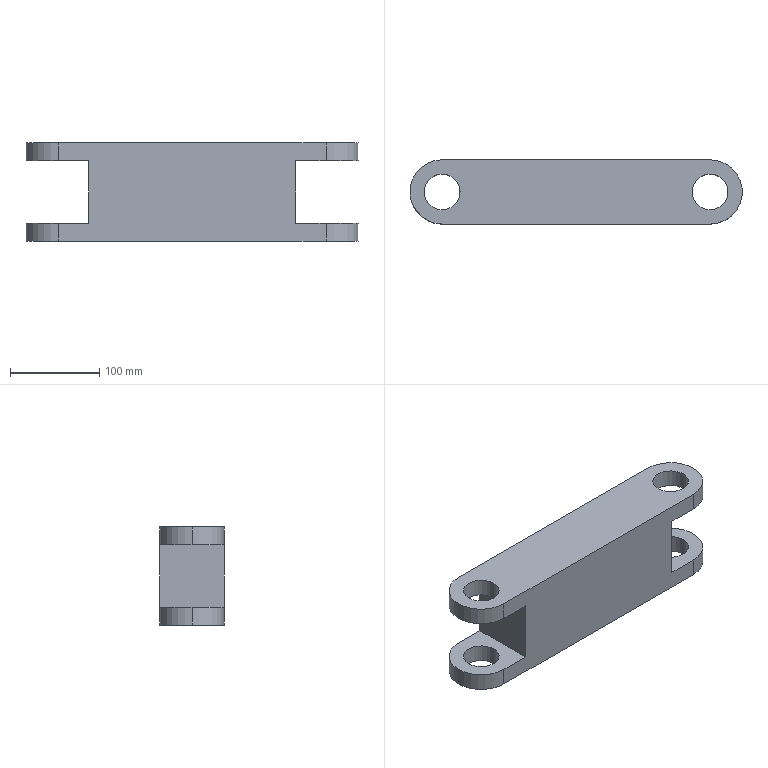Part | SolidWorks | 1 solid | 24 faces | box 372 x 72 x 110 mm | volume 2095609 mm3 | cylinder 14 | plane 10 | commonest cylinder face diameters 40 x8 72 x6
STEP:
#1=CARTESIAN_POINT('',(320.,0.,-35.));
#2=VERTEX_POINT('',#1);
#3=CARTESIAN_POINT('',(280.,0.,-35.));
#4=VERTEX_POINT('',#3);
#5=CARTESIAN_POINT('',(300.,0.,-35.));
#6=DIRECTION('',(0.,0.,-1.));
#7=DIRECTION('',(-1.,0.,0.));
#8=AXIS2_PLACEMENT_3D('',#5,#6,#7);
#9=CIRCLE('',#8,20.);
#10=EDGE_CURVE('',#2,#4,#9,.T.);
#11=ORIENTED_EDGE('',*,*,#10,.F.);
#12=CARTESIAN_POINT('',(320.,0.,-55.));
#13=VERTEX_POINT('',#12);
#14=CARTESIAN_POINT('',(320.,0.,55.));
#15=DIRECTION('',(0.,0.,-1.));
#16=VECTOR('',#15,1000.);
#17=LINE('',#14,#16);
#18=EDGE_CURVE('',#2,#13,#17,.T.);
#19=ORIENTED_EDGE('',*,*,#18,.T.);
#20=CARTESIAN_POINT('',(280.,0.,-55.));
#21=VERTEX_POINT('',#20);
#22=CARTESIAN_POINT('',(300.,0.,-55.));
#23=DIRECTION('',(0.,0.,1.));
#24=DIRECTION('',(1.,0.,0.));
#25=AXIS2_PLACEMENT_3D('',#22,#23,#24);
#26=CIRCLE('',#25,20.);
#27=EDGE_CURVE('',#21,#13,#26,.T.);
#28=ORIENTED_EDGE('',*,*,#27,.F.);
#29=CARTESIAN_POINT('',(280.,0.,55.));
#30=DIRECTION('',(0.,0.,-1.));
#31=VECTOR('',#30,1000.);
#32=LINE('',#29,#31);
#33=EDGE_CURVE('',#4,#21,#32,.T.);
#34=ORIENTED_EDGE('',*,*,#33,.F.);
#35=EDGE_LOOP('',(#11,#19,#28,#34));
#36=FACE_OUTER_BOUND('',#35,.T.);
#37=CARTESIAN_POINT('',(300.,0.,55.));
#38=DIRECTION('',(0.,0.,-1.));
#39=DIRECTION('',(-1.,0.,0.));
#40=AXIS2_PLACEMENT_3D('',#37,#38,#39);
#41=CYLINDRICAL_SURFACE('',#40,20.);
#42=ADVANCED_FACE('',(#36),#41,.F.);
#43=CARTESIAN_POINT('',(20.,0.,-35.));
#44=VERTEX_POINT('',#43);
#45=CARTESIAN_POINT('',(-20.,0.,-35.));
#46=VERTEX_POINT('',#45);
#47=CARTESIAN_POINT('',(0.,0.,-35.));
#48=DIRECTION('',(0.,0.,-1.));
#49=DIRECTION('',(-1.,0.,0.));
#50=AXIS2_PLACEMENT_3D('',#47,#48,#49);
#51=CIRCLE('',#50,20.);
#52=EDGE_CURVE('',#44,#46,#51,.T.);
#53=ORIENTED_EDGE('',*,*,#52,.F.);
#54=CARTESIAN_POINT('',(20.,0.,-55.));
#55=VERTEX_POINT('',#54);
#56=CARTESIAN_POINT('',(20.,0.,55.));
#57=DIRECTION('',(0.,0.,-1.));
#58=VECTOR('',#57,1000.);
#59=LINE('',#56,#58);
#60=EDGE_CURVE('',#44,#55,#59,.T.);
#61=ORIENTED_EDGE('',*,*,#60,.T.);
#62=CARTESIAN_POINT('',(-20.,0.,-55.));
#63=VERTEX_POINT('',#62);
#64=CARTESIAN_POINT('',(0.,0.,-55.));
#65=DIRECTION('',(0.,0.,1.));
#66=DIRECTION('',(1.,0.,0.));
#67=AXIS2_PLACEMENT_3D('',#64,#65,#66);
#68=CIRCLE('',#67,20.);
#69=EDGE_CURVE('',#63,#55,#68,.T.);
#70=ORIENTED_EDGE('',*,*,#69,.F.);
#71=CARTESIAN_POINT('',(-20.,0.,55.));
#72=DIRECTION('',(0.,0.,-1.));
#73=VECTOR('',#72,1000.);
#74=LINE('',#71,#73);
#75=EDGE_CURVE('',#46,#63,#74,.T.);
#76=ORIENTED_EDGE('',*,*,#75,.F.);
#77=EDGE_LOOP('',(#53,#61,#70,#76));
#78=FACE_OUTER_BOUND('',#77,.T.);
#79=CARTESIAN_POINT('',(0.,0.,55.));
#80=DIRECTION('',(0.,0.,-1.));
#81=DIRECTION('',(-1.,0.,0.));
#82=AXIS2_PLACEMENT_3D('',#79,#80,#81);
#83=CYLINDRICAL_SURFACE('',#82,20.);
#84=ADVANCED_FACE('',(#78),#83,.F.);
#85=CARTESIAN_POINT('',(0.,-36.,-35.));
#86=VERTEX_POINT('',#85);
#87=CARTESIAN_POINT('',(-36.,0.,-35.));
#88=VERTEX_POINT('',#87);
#89=CARTESIAN_POINT('',(0.,0.,-35.));
#90=DIRECTION('',(0.,0.,-1.));
#91=DIRECTION('',(-1.,0.,0.));
#92=AXIS2_PLACEMENT_3D('',#89,#90,#91);
#93=CIRCLE('',#92,36.);
#94=EDGE_CURVE('',#86,#88,#93,.T.);
#95=ORIENTED_EDGE('',*,*,#94,.T.);
#96=CARTESIAN_POINT('',(-36.,0.,-55.));
#97=VERTEX_POINT('',#96);
#98=CARTESIAN_POINT('',(-36.,0.,55.));
#99=DIRECTION('',(0.,0.,-1.));
#100=VECTOR('',#99,1000.);
#101=LINE('',#98,#100);
#102=EDGE_CURVE('',#88,#97,#101,.T.);
#103=ORIENTED_EDGE('',*,*,#102,.T.);
#104=CARTESIAN_POINT('',(0.,-36.,-55.));
#105=VERTEX_POINT('',#104);
#106=CARTESIAN_POINT('',(0.,0.,-55.));
#107=DIRECTION('',(0.,0.,1.));
#108=DIRECTION('',(1.,0.,0.));
#109=AXIS2_PLACEMENT_3D('',#106,#107,#108);
#110=CIRCLE('',#109,36.);
#111=EDGE_CURVE('',#97,#105,#110,.T.);
#112=ORIENTED_EDGE('',*,*,#111,.T.);
#113=CARTESIAN_POINT('',(0.,-36.,55.));
#114=DIRECTION('',(0.,0.,-1.));
#115=VECTOR('',#114,1000.);
#116=LINE('',#113,#115);
#117=EDGE_CURVE('',#86,#105,#116,.T.);
#118=ORIENTED_EDGE('',*,*,#117,.F.);
#119=EDGE_LOOP('',(#95,#103,#112,#118));
#120=FACE_OUTER_BOUND('',#119,.T.);
#121=CARTESIAN_POINT('',(0.,0.,55.));
#122=DIRECTION('',(0.,0.,-1.));
#123=DIRECTION('',(-1.,0.,0.));
#124=AXIS2_PLACEMENT_3D('',#121,#122,#123);
#125=CYLINDRICAL_SURFACE('',#124,36.);
#126=ADVANCED_FACE('',(#120),#125,.T.);
#127=CARTESIAN_POINT('',(280.,0.,55.));
#128=VERTEX_POINT('',#127);
#129=CARTESIAN_POINT('',(320.,0.,55.));
#130=VERTEX_POINT('',#129);
#131=CARTESIAN_POINT('',(300.,0.,55.));
#132=DIRECTION('',(0.,0.,1.));
#133=DIRECTION('',(1.,0.,0.));
#134=AXIS2_PLACEMENT_3D('',#131,#132,#133);
#135=CIRCLE('',#134,20.);
#136=EDGE_CURVE('',#128,#130,#135,.T.);
#137=ORIENTED_EDGE('',*,*,#136,.T.);
#138=CARTESIAN_POINT('',(320.,0.,35.));
#139=VERTEX_POINT('',#138);
#140=CARTESIAN_POINT('',(320.,0.,55.));
#141=DIRECTION('',(0.,0.,-1.));
#142=VECTOR('',#141,1000.);
#143=LINE('',#140,#142);
#144=EDGE_CURVE('',#130,#139,#143,.T.);
#145=ORIENTED_EDGE('',*,*,#144,.T.);
#146=CARTESIAN_POINT('',(280.,0.,35.));
#147=VERTEX_POINT('',#146);
#148=CARTESIAN_POINT('',(300.,0.,35.));
#149=DIRECTION('',(0.,0.,1.));
#150=DIRECTION('',(1.,0.,0.));
#151=AXIS2_PLACEMENT_3D('',#148,#149,#150);
#152=CIRCLE('',#151,20.);
#153=EDGE_CURVE('',#147,#139,#152,.T.);
#154=ORIENTED_EDGE('',*,*,#153,.F.);
#155=CARTESIAN_POINT('',(280.,0.,55.));
#156=DIRECTION('',(0.,0.,-1.));
#157=VECTOR('',#156,1000.);
#158=LINE('',#155,#157);
#159=EDGE_CURVE('',#128,#147,#158,.T.);
#160=ORIENTED_EDGE('',*,*,#159,.F.);
#161=EDGE_LOOP('',(#137,#145,#154,#160));
#162=FACE_OUTER_BOUND('',#161,.T.);
#163=CARTESIAN_POINT('',(300.,0.,55.));
#164=DIRECTION('',(0.,0.,-1.));
#165=DIRECTION('',(-1.,0.,0.));
#166=AXIS2_PLACEMENT_3D('',#163,#164,#165);
#167=CYLINDRICAL_SURFACE('',#166,20.);
#168=ADVANCED_FACE('',(#162),#167,.F.);
#169=CARTESIAN_POINT('',(-20.,0.,55.));
#170=VERTEX_POINT('',#169);
#171=CARTESIAN_POINT('',(20.,0.,55.));
#172=VERTEX_POINT('',#171);
#173=CARTESIAN_POINT('',(0.,0.,55.));
#174=DIRECTION('',(0.,0.,1.));
#175=DIRECTION('',(1.,0.,0.));
#176=AXIS2_PLACEMENT_3D('',#173,#174,#175);
#177=CIRCLE('',#176,20.);
#178=EDGE_CURVE('',#170,#172,#177,.T.);
#179=ORIENTED_EDGE('',*,*,#178,.T.);
#180=CARTESIAN_POINT('',(20.,0.,35.));
#181=VERTEX_POINT('',#180);
#182=CARTESIAN_POINT('',(20.,0.,55.));
#183=DIRECTION('',(0.,0.,-1.));
#184=VECTOR('',#183,1000.);
#185=LINE('',#182,#184);
#186=EDGE_CURVE('',#172,#181,#185,.T.);
#187=ORIENTED_EDGE('',*,*,#186,.T.);
#188=CARTESIAN_POINT('',(-20.,0.,35.));
#189=VERTEX_POINT('',#188);
#190=CARTESIAN_POINT('',(0.,0.,35.));
#191=DIRECTION('',(0.,0.,1.));
#192=DIRECTION('',(1.,0.,0.));
#193=AXIS2_PLACEMENT_3D('',#190,#191,#192);
#194=CIRCLE('',#193,20.);
#195=EDGE_CURVE('',#189,#181,#194,.T.);
#196=ORIENTED_EDGE('',*,*,#195,.F.);
#197=CARTESIAN_POINT('',(-20.,0.,55.));
#198=DIRECTION('',(0.,0.,-1.));
#199=VECTOR('',#198,1000.);
#200=LINE('',#197,#199);
#201=EDGE_CURVE('',#170,#189,#200,.T.);
#202=ORIENTED_EDGE('',*,*,#201,.F.);
#203=EDGE_LOOP('',(#179,#187,#196,#202));
#204=FACE_OUTER_BOUND('',#203,.T.);
#205=CARTESIAN_POINT('',(0.,0.,55.));
#206=DIRECTION('',(0.,0.,-1.));
#207=DIRECTION('',(-1.,0.,0.));
#208=AXIS2_PLACEMENT_3D('',#205,#206,#207);
#209=CYLINDRICAL_SURFACE('',#208,20.);
#210=ADVANCED_FACE('',(#204),#209,.F.);
#211=CARTESIAN_POINT('',(-36.,0.,55.));
#212=VERTEX_POINT('',#211);
#213=CARTESIAN_POINT('',(0.,-36.,55.));
#214=VERTEX_POINT('',#213);
#215=CARTESIAN_POINT('',(0.,0.,55.));
#216=DIRECTION('',(0.,0.,1.));
#217=DIRECTION('',(1.,0.,0.));
#218=AXIS2_PLACEMENT_3D('',#215,#216,#217);
#219=CIRCLE('',#218,36.);
#220=EDGE_CURVE('',#212,#214,#219,.T.);
#221=ORIENTED_EDGE('',*,*,#220,.F.);
#222=CARTESIAN_POINT('',(-36.,0.,35.));
#223=VERTEX_POINT('',#222);
#224=CARTESIAN_POINT('',(-36.,0.,55.));
#225=DIRECTION('',(0.,0.,-1.));
#226=VECTOR('',#225,1000.);
#227=LINE('',#224,#226);
#228=EDGE_CURVE('',#212,#223,#227,.T.);
#229=ORIENTED_EDGE('',*,*,#228,.T.);
#230=CARTESIAN_POINT('',(0.,-36.,35.));
#231=VERTEX_POINT('',#230);
#232=CARTESIAN_POINT('',(0.,0.,35.));
#233=DIRECTION('',(0.,0.,1.));
#234=DIRECTION('',(1.,0.,0.));
#235=AXIS2_PLACEMENT_3D('',#232,#233,#234);
#236=CIRCLE('',#235,36.);
#237=EDGE_CURVE('',#223,#231,#236,.T.);
#238=ORIENTED_EDGE('',*,*,#237,.T.);
#239=CARTESIAN_POINT('',(0.,-36.,55.));
#240=DIRECTION('',(0.,0.,-1.));
#241=VECTOR('',#240,1000.);
#242=LINE('',#239,#241);
#243=EDGE_CURVE('',#214,#231,#242,.T.);
#244=ORIENTED_EDGE('',*,*,#243,.F.);
#245=EDGE_LOOP('',(#221,#229,#238,#244));
#246=FACE_OUTER_BOUND('',#245,.T.);
#247=CARTESIAN_POINT('',(0.,0.,55.));
#248=DIRECTION('',(0.,0.,-1.));
#249=DIRECTION('',(-1.,0.,0.));
#250=AXIS2_PLACEMENT_3D('',#247,#248,#249);
#251=CYLINDRICAL_SURFACE('',#250,36.);
#252=ADVANCED_FACE('',(#246),#251,.T.);
#253=ORIENTED_EDGE('',*,*,#228,.F.);
#254=CARTESIAN_POINT('',(0.,36.,55.));
#255=VERTEX_POINT('',#254);
#256=CARTESIAN_POINT('',(0.,0.,55.));
#257=DIRECTION('',(0.,0.,1.));
#258=DIRECTION('',(1.,0.,0.));
#259=AXIS2_PLACEMENT_3D('',#256,#257,#258);
#260=CIRCLE('',#259,36.);
#261=EDGE_CURVE('',#255,#212,#260,.T.);
#262=ORIENTED_EDGE('',*,*,#261,.F.);
#263=CARTESIAN_POINT('',(0.,36.,35.));
#264=VERTEX_POINT('',#263);
#265=CARTESIAN_POINT('',(0.,36.,55.));
#266=DIRECTION('',(0.,0.,-1.));
#267=VECTOR('',#266,1000.);
#268=LINE('',#265,#267);
#269=EDGE_CURVE('',#255,#264,#268,.T.);
#270=ORIENTED_EDGE('',*,*,#269,.T.);
#271=CARTESIAN_POINT('',(0.,0.,35.));
#272=DIRECTION('',(0.,0.,1.));
#273=DIRECTION('',(1.,0.,0.));
#274=AXIS2_PLACEMENT_3D('',#271,#272,#273);
#275=CIRCLE('',#274,36.);
#276=EDGE_CURVE('',#264,#223,#275,.T.);
#277=ORIENTED_EDGE('',*,*,#276,.T.);
#278=EDGE_LOOP('',(#253,#262,#270,#277));
#279=FACE_OUTER_BOUND('',#278,.T.);
#280=CARTESIAN_POINT('',(0.,0.,55.));
#281=DIRECTION('',(0.,0.,-1.));
#282=DIRECTION('',(-1.,0.,0.));
#283=AXIS2_PLACEMENT_3D('',#280,#281,#282);
#284=CYLINDRICAL_SURFACE('',#283,36.);
#285=ADVANCED_FACE('',(#279),#284,.T.);
#286=CARTESIAN_POINT('',(300.,-36.,55.));
#287=VERTEX_POINT('',#286);
#288=CARTESIAN_POINT('',(300.,-36.,35.));
#289=VERTEX_POINT('',#288);
#290=CARTESIAN_POINT('',(300.,-36.,55.));
#291=DIRECTION('',(0.,0.,-1.));
#292=VECTOR('',#291,1000.);
#293=LINE('',#290,#292);
#294=EDGE_CURVE('',#287,#289,#293,.T.);
#295=ORIENTED_EDGE('',*,*,#294,.T.);
#296=CARTESIAN_POINT('',(300.,36.,35.));
#297=VERTEX_POINT('',#296);
#298=CARTESIAN_POINT('',(300.,0.,35.));
#299=DIRECTION('',(0.,0.,1.));
#300=DIRECTION('',(1.,0.,0.));
#301=AXIS2_PLACEMENT_3D('',#298,#299,#300);
#302=CIRCLE('',#301,36.);
#303=EDGE_CURVE('',#289,#297,#302,.T.);
#304=ORIENTED_EDGE('',*,*,#303,.T.);
#305=CARTESIAN_POINT('',(300.,36.,55.));
#306=VERTEX_POINT('',#305);
#307=CARTESIAN_POINT('',(300.,36.,55.));
#308=DIRECTION('',(0.,0.,-1.));
#309=VECTOR('',#308,1000.);
#310=LINE('',#307,#309);
#311=EDGE_CURVE('',#306,#297,#310,.T.);
#312=ORIENTED_EDGE('',*,*,#311,.F.);
#313=CARTESIAN_POINT('',(300.,0.,55.));
#314=DIRECTION('',(0.,0.,1.));
#315=DIRECTION('',(1.,0.,0.));
#316=AXIS2_PLACEMENT_3D('',#313,#314,#315);
#317=CIRCLE('',#316,36.);
#318=EDGE_CURVE('',#287,#306,#317,.T.);
#319=ORIENTED_EDGE('',*,*,#318,.F.);
#320=EDGE_LOOP('',(#295,#304,#312,#319));
#321=FACE_OUTER_BOUND('',#320,.T.);
#322=CARTESIAN_POINT('',(300.,0.,55.));
#323=DIRECTION('',(0.,0.,-1.));
#324=DIRECTION('',(-1.,0.,0.));
#325=AXIS2_PLACEMENT_3D('',#322,#323,#324);
#326=CYLINDRICAL_SURFACE('',#325,36.);
#327=ADVANCED_FACE('',(#321),#326,.T.);
#328=ORIENTED_EDGE('',*,*,#186,.F.);
#329=CARTESIAN_POINT('',(0.,0.,55.));
#330=DIRECTION('',(0.,0.,1.));
#331=DIRECTION('',(1.,0.,0.));
#332=AXIS2_PLACEMENT_3D('',#329,#330,#331);
#333=CIRCLE('',#332,20.);
#334=EDGE_CURVE('',#172,#170,#333,.T.);
#335=ORIENTED_EDGE('',*,*,#334,.T.);
#336=ORIENTED_EDGE('',*,*,#201,.T.);
#337=CARTESIAN_POINT('',(0.,0.,35.));
#338=DIRECTION('',(0.,0.,1.));
#339=DIRECTION('',(1.,0.,0.));
#340=AXIS2_PLACEMENT_3D('',#337,#338,#339);
#341=CIRCLE('',#340,20.);
#342=EDGE_CURVE('',#181,#189,#341,.T.);
#343=ORIENTED_EDGE('',*,*,#342,.F.);
#344=EDGE_LOOP('',(#328,#335,#336,#343));
#345=FACE_OUTER_BOUND('',#344,.T.);
#346=CARTESIAN_POINT('',(0.,0.,55.));
#347=DIRECTION('',(0.,0.,-1.));
#348=DIRECTION('',(-1.,0.,0.));
#349=AXIS2_PLACEMENT_3D('',#346,#347,#348);
#350=CYLINDRICAL_SURFACE('',#349,20.);
#351=ADVANCED_FACE('',(#345),#350,.F.);
#352=ORIENTED_EDGE('',*,*,#144,.F.);
#353=CARTESIAN_POINT('',(300.,0.,55.));
#354=DIRECTION('',(0.,0.,1.));
#355=DIRECTION('',(1.,0.,0.));
#356=AXIS2_PLACEMENT_3D('',#353,#354,#355);
#357=CIRCLE('',#356,20.);
#358=EDGE_CURVE('',#130,#128,#357,.T.);
#359=ORIENTED_EDGE('',*,*,#358,.T.);
#360=ORIENTED_EDGE('',*,*,#159,.T.);
#361=CARTESIAN_POINT('',(300.,0.,35.));
#362=DIRECTION('',(0.,0.,1.));
#363=DIRECTION('',(1.,0.,0.));
#364=AXIS2_PLACEMENT_3D('',#361,#362,#363);
#365=CIRCLE('',#364,20.);
#366=EDGE_CURVE('',#139,#147,#365,.T.);
#367=ORIENTED_EDGE('',*,*,#366,.F.);
#368=EDGE_LOOP('',(#352,#359,#360,#367));
#369=FACE_OUTER_BOUND('',#368,.T.);
#370=CARTESIAN_POINT('',(300.,0.,55.));
#371=DIRECTION('',(0.,0.,-1.));
#372=DIRECTION('',(-1.,0.,0.));
#373=AXIS2_PLACEMENT_3D('',#370,#371,#372);
#374=CYLINDRICAL_SURFACE('',#373,20.);
#375=ADVANCED_FACE('',(#369),#374,.F.);
#376=ORIENTED_EDGE('',*,*,#178,.F.);
#377=ORIENTED_EDGE('',*,*,#334,.F.);
#378=EDGE_LOOP('',(#376,#377));
#379=FACE_BOUND('',#378,.T.);
#380=ORIENTED_EDGE('',*,*,#261,.T.);
#381=ORIENTED_EDGE('',*,*,#220,.T.);
#382=CARTESIAN_POINT('',(0.,-36.,55.));
#383=DIRECTION('',(1.,0.,0.));
#384=VECTOR('',#383,1000.);
#385=LINE('',#382,#384);
#386=EDGE_CURVE('',#214,#287,#385,.T.);
#387=ORIENTED_EDGE('',*,*,#386,.T.);
#388=ORIENTED_EDGE('',*,*,#318,.T.);
#389=CARTESIAN_POINT('',(0.,36.,55.));
#390=DIRECTION('',(-1.,0.,0.));
#391=VECTOR('',#390,1000.);
#392=LINE('',#389,#391);
#393=EDGE_CURVE('',#306,#255,#392,.T.);
#394=ORIENTED_EDGE('',*,*,#393,.T.);
#395=EDGE_LOOP('',(#380,#381,#387,#388,#394));
#396=FACE_OUTER_BOUND('',#395,.T.);
#397=ORIENTED_EDGE('',*,*,#136,.F.);
#398=ORIENTED_EDGE('',*,*,#358,.F.);
#399=EDGE_LOOP('',(#397,#398));
#400=FACE_BOUND('',#399,.T.);
#401=CARTESIAN_POINT('',(0.,0.,55.));
#402=DIRECTION('',(0.,0.,1.));
#403=DIRECTION('',(1.,0.,0.));
#404=AXIS2_PLACEMENT_3D('',#401,#402,#403);
#405=PLANE('',#404);
#406=ADVANCED_FACE('',(#379,#396,#400),#405,.T.);
#407=CARTESIAN_POINT('',(0.,36.,-55.));
#408=VERTEX_POINT('',#407);
#409=CARTESIAN_POINT('',(0.,0.,-55.));
#410=DIRECTION('',(0.,0.,1.));
#411=DIRECTION('',(1.,0.,0.));
#412=AXIS2_PLACEMENT_3D('',#409,#410,#411);
#413=CIRCLE('',#412,36.);
#414=EDGE_CURVE('',#408,#97,#413,.T.);
#415=ORIENTED_EDGE('',*,*,#414,.F.);
#416=CARTESIAN_POINT('',(300.,36.,-55.));
#417=VERTEX_POINT('',#416);
#418=CARTESIAN_POINT('',(0.,36.,-55.));
#419=DIRECTION('',(-1.,0.,0.));
#420=VECTOR('',#419,1000.);
#421=LINE('',#418,#420);
#422=EDGE_CURVE('',#417,#408,#421,.T.);
#423=ORIENTED_EDGE('',*,*,#422,.F.);
#424=CARTESIAN_POINT('',(300.,-36.,-55.));
#425=VERTEX_POINT('',#424);
#426=CARTESIAN_POINT('',(300.,0.,-55.));
#427=DIRECTION('',(0.,0.,1.));
#428=DIRECTION('',(1.,0.,0.));
#429=AXIS2_PLACEMENT_3D('',#426,#427,#428);
#430=CIRCLE('',#429,36.);
#431=EDGE_CURVE('',#425,#417,#430,.T.);
#432=ORIENTED_EDGE('',*,*,#431,.F.);
#433=CARTESIAN_POINT('',(0.,-36.,-55.));
#434=DIRECTION('',(1.,0.,0.));
#435=VECTOR('',#434,1000.);
#436=LINE('',#433,#435);
#437=EDGE_CURVE('',#105,#425,#436,.T.);
#438=ORIENTED_EDGE('',*,*,#437,.F.);
#439=ORIENTED_EDGE('',*,*,#111,.F.);
#440=EDGE_LOOP('',(#415,#423,#432,#438,#439));
#441=FACE_OUTER_BOUND('',#440,.T.);
#442=ORIENTED_EDGE('',*,*,#69,.T.);
#443=CARTESIAN_POINT('',(0.,0.,-55.));
#444=DIRECTION('',(0.,0.,1.));
#445=DIRECTION('',(1.,0.,0.));
#446=AXIS2_PLACEMENT_3D('',#443,#444,#445);
#447=CIRCLE('',#446,20.);
#448=EDGE_CURVE('',#55,#63,#447,.T.);
#449=ORIENTED_EDGE('',*,*,#448,.T.);
#450=EDGE_LOOP('',(#442,#449));
#451=FACE_BOUND('',#450,.T.);
#452=ORIENTED_EDGE('',*,*,#27,.T.);
#453=CARTESIAN_POINT('',(300.,0.,-55.));
#454=DIRECTION('',(0.,0.,1.));
#455=DIRECTION('',(1.,0.,0.));
#456=AXIS2_PLACEMENT_3D('',#453,#454,#455);
#457=CIRCLE('',#456,20.);
#458=EDGE_CURVE('',#13,#21,#457,.T.);
#459=ORIENTED_EDGE('',*,*,#458,.T.);
#460=EDGE_LOOP('',(#452,#459));
#461=FACE_BOUND('',#460,.T.);
#462=CARTESIAN_POINT('',(0.,0.,-55.));
#463=DIRECTION('',(0.,0.,1.));
#464=DIRECTION('',(1.,0.,0.));
#465=AXIS2_PLACEMENT_3D('',#462,#463,#464);
#466=PLANE('',#465);
#467=ADVANCED_FACE('',(#441,#451,#461),#466,.F.);
#468=ORIENTED_EDGE('',*,*,#102,.F.);
#469=CARTESIAN_POINT('',(0.,36.,-35.));
#470=VERTEX_POINT('',#469);
#471=CARTESIAN_POINT('',(0.,0.,-35.));
#472=DIRECTION('',(0.,0.,-1.));
#473=DIRECTION('',(-1.,0.,0.));
#474=AXIS2_PLACEMENT_3D('',#471,#472,#473);
#475=CIRCLE('',#474,36.);
#476=EDGE_CURVE('',#88,#470,#475,.T.);
#477=ORIENTED_EDGE('',*,*,#476,.T.);
#478=CARTESIAN_POINT('',(0.,36.,55.));
#479=DIRECTION('',(0.,0.,-1.));
#480=VECTOR('',#479,1000.);
#481=LINE('',#478,#480);
#482=EDGE_CURVE('',#470,#408,#481,.T.);
#483=ORIENTED_EDGE('',*,*,#482,.T.);
#484=ORIENTED_EDGE('',*,*,#414,.T.);
#485=EDGE_LOOP('',(#468,#477,#483,#484));
#486=FACE_OUTER_BOUND('',#485,.T.);
#487=CARTESIAN_POINT('',(0.,0.,55.));
#488=DIRECTION('',(0.,0.,-1.));
#489=DIRECTION('',(-1.,0.,0.));
#490=AXIS2_PLACEMENT_3D('',#487,#488,#489);
#491=CYLINDRICAL_SURFACE('',#490,36.);
#492=ADVANCED_FACE('',(#486),#491,.T.);
#493=ORIENTED_EDGE('',*,*,#243,.T.);
#494=CARTESIAN_POINT('',(34.,-36.,35.));
#495=VERTEX_POINT('',#494);
#496=CARTESIAN_POINT('',(0.,-36.,35.));
#497=DIRECTION('',(1.,0.,0.));
#498=VECTOR('',#497,1000.);
#499=LINE('',#496,#498);
#500=EDGE_CURVE('',#231,#495,#499,.T.);
#501=ORIENTED_EDGE('',*,*,#500,.T.);
#502=CARTESIAN_POINT('',(34.,-36.,-35.));
#503=VERTEX_POINT('',#502);
#504=CARTESIAN_POINT('',(34.,-36.,55.));
#505=DIRECTION('',(0.,0.,-1.));
#506=VECTOR('',#505,1000.);
#507=LINE('',#504,#506);
#508=EDGE_CURVE('',#495,#503,#507,.T.);
#509=ORIENTED_EDGE('',*,*,#508,.T.);
#510=CARTESIAN_POINT('',(0.,-36.,-35.));
#511=DIRECTION('',(-1.,0.,0.));
#512=VECTOR('',#511,1000.);
#513=LINE('',#510,#512);
#514=EDGE_CURVE('',#503,#86,#513,.T.);
#515=ORIENTED_EDGE('',*,*,#514,.T.);
#516=ORIENTED_EDGE('',*,*,#117,.T.);
#517=ORIENTED_EDGE('',*,*,#437,.T.);
#518=CARTESIAN_POINT('',(300.,-36.,-35.));
#519=VERTEX_POINT('',#518);
#520=CARTESIAN_POINT('',(300.,-36.,55.));
#521=DIRECTION('',(0.,0.,-1.));
#522=VECTOR('',#521,1000.);
#523=LINE('',#520,#522);
#524=EDGE_CURVE('',#519,#425,#523,.T.);
#525=ORIENTED_EDGE('',*,*,#524,.F.);
#526=CARTESIAN_POINT('',(266.,-36.,-35.));
#527=VERTEX_POINT('',#526);
#528=CARTESIAN_POINT('',(0.,-36.,-35.));
#529=DIRECTION('',(-1.,0.,0.));
#530=VECTOR('',#529,1000.);
#531=LINE('',#528,#530);
#532=EDGE_CURVE('',#519,#527,#531,.T.);
#533=ORIENTED_EDGE('',*,*,#532,.T.);
#534=CARTESIAN_POINT('',(266.,-36.,35.));
#535=VERTEX_POINT('',#534);
#536=CARTESIAN_POINT('',(266.,-36.,55.));
#537=DIRECTION('',(0.,0.,1.));
#538=VECTOR('',#537,1000.);
#539=LINE('',#536,#538);
#540=EDGE_CURVE('',#527,#535,#539,.T.);
#541=ORIENTED_EDGE('',*,*,#540,.T.);
#542=CARTESIAN_POINT('',(0.,-36.,35.));
#543=DIRECTION('',(1.,0.,0.));
#544=VECTOR('',#543,1000.);
#545=LINE('',#542,#544);
#546=EDGE_CURVE('',#535,#289,#545,.T.);
#547=ORIENTED_EDGE('',*,*,#546,.T.);
#548=ORIENTED_EDGE('',*,*,#294,.F.);
#549=ORIENTED_EDGE('',*,*,#386,.F.);
#550=EDGE_LOOP('',(#493,#501,#509,#515,#516,#517,#525,#533,#541,#547,#548,#549));
#551=FACE_OUTER_BOUND('',#550,.T.);
#552=CARTESIAN_POINT('',(0.,-36.,55.));
#553=DIRECTION('',(0.,1.,0.));
#554=DIRECTION('',(-1.,0.,0.));
#555=AXIS2_PLACEMENT_3D('',#552,#553,#554);
#556=PLANE('',#555);
#557=ADVANCED_FACE('',(#551),#556,.F.);
#558=CARTESIAN_POINT('',(300.,36.,-35.));
#559=VERTEX_POINT('',#558);
#560=CARTESIAN_POINT('',(300.,36.,55.));
#561=DIRECTION('',(0.,0.,-1.));
#562=VECTOR('',#561,1000.);
#563=LINE('',#560,#562);
#564=EDGE_CURVE('',#559,#417,#563,.T.);
#565=ORIENTED_EDGE('',*,*,#564,.F.);
#566=CARTESIAN_POINT('',(300.,0.,-35.));
#567=DIRECTION('',(0.,0.,-1.));
#568=DIRECTION('',(-1.,0.,0.));
#569=AXIS2_PLACEMENT_3D('',#566,#567,#568);
#570=CIRCLE('',#569,36.);
#571=EDGE_CURVE('',#559,#519,#570,.T.);
#572=ORIENTED_EDGE('',*,*,#571,.T.);
#573=ORIENTED_EDGE('',*,*,#524,.T.);
#574=ORIENTED_EDGE('',*,*,#431,.T.);
#575=EDGE_LOOP('',(#565,#572,#573,#574));
#576=FACE_OUTER_BOUND('',#575,.T.);
#577=CARTESIAN_POINT('',(300.,0.,55.));
#578=DIRECTION('',(0.,0.,-1.));
#579=DIRECTION('',(-1.,0.,0.));
#580=AXIS2_PLACEMENT_3D('',#577,#578,#579);
#581=CYLINDRICAL_SURFACE('',#580,36.);
#582=ADVANCED_FACE('',(#576),#581,.T.);
#583=CARTESIAN_POINT('',(34.,36.,35.));
#584=VERTEX_POINT('',#583);
#585=CARTESIAN_POINT('',(34.,36.,-35.));
#586=VERTEX_POINT('',#585);
#587=CARTESIAN_POINT('',(34.,36.,-35.));
#588=DIRECTION('',(0.,0.,-1.));
#589=VECTOR('',#588,1000.);
#590=LINE('',#587,#589);
#591=EDGE_CURVE('',#584,#586,#590,.T.);
#592=ORIENTED_EDGE('',*,*,#591,.F.);
#593=CARTESIAN_POINT('',(-106.,36.,35.));
#594=DIRECTION('',(1.,0.,0.));
#595=VECTOR('',#594,1000.);
#596=LINE('',#593,#595);
#597=EDGE_CURVE('',#264,#584,#596,.T.);
#598=ORIENTED_EDGE('',*,*,#597,.F.);
#599=ORIENTED_EDGE('',*,*,#269,.F.);
#600=ORIENTED_EDGE('',*,*,#393,.F.);
#601=ORIENTED_EDGE('',*,*,#311,.T.);
#602=CARTESIAN_POINT('',(266.,36.,35.));
#603=VERTEX_POINT('',#602);
#604=CARTESIAN_POINT('',(406.,36.,35.));
#605=DIRECTION('',(1.,0.,0.));
#606=VECTOR('',#605,1000.);
#607=LINE('',#604,#606);
#608=EDGE_CURVE('',#603,#297,#607,.T.);
#609=ORIENTED_EDGE('',*,*,#608,.F.);
#610=CARTESIAN_POINT('',(266.,36.,-35.));
#611=VERTEX_POINT('',#610);
#612=CARTESIAN_POINT('',(266.,36.,-35.));
#613=DIRECTION('',(0.,0.,1.));
#614=VECTOR('',#613,1000.);
#615=LINE('',#612,#614);
#616=EDGE_CURVE('',#611,#603,#615,.T.);
#617=ORIENTED_EDGE('',*,*,#616,.F.);
#618=CARTESIAN_POINT('',(406.,36.,-35.));
#619=DIRECTION('',(-1.,0.,0.));
#620=VECTOR('',#619,1000.);
#621=LINE('',#618,#620);
#622=EDGE_CURVE('',#559,#611,#621,.T.);
#623=ORIENTED_EDGE('',*,*,#622,.F.);
#624=ORIENTED_EDGE('',*,*,#564,.T.);
#625=ORIENTED_EDGE('',*,*,#422,.T.);
#626=ORIENTED_EDGE('',*,*,#482,.F.);
#627=CARTESIAN_POINT('',(-106.,36.,-35.));
#628=DIRECTION('',(-1.,0.,0.));
#629=VECTOR('',#628,1000.);
#630=LINE('',#627,#629);
#631=EDGE_CURVE('',#586,#470,#630,.T.);
#632=ORIENTED_EDGE('',*,*,#631,.F.);
#633=EDGE_LOOP('',(#592,#598,#599,#600,#601,#609,#617,#623,#624,#625,#626,#632));
#634=FACE_OUTER_BOUND('',#633,.T.);
#635=CARTESIAN_POINT('',(0.,36.,55.));
#636=DIRECTION('',(0.,-1.,0.));
#637=DIRECTION('',(1.,0.,0.));
#638=AXIS2_PLACEMENT_3D('',#635,#636,#637);
#639=PLANE('',#638);
#640=ADVANCED_FACE('',(#634),#639,.F.);
#641=ORIENTED_EDGE('',*,*,#60,.F.);
#642=CARTESIAN_POINT('',(0.,0.,-35.));
#643=DIRECTION('',(0.,0.,-1.));
#644=DIRECTION('',(-1.,0.,0.));
#645=AXIS2_PLACEMENT_3D('',#642,#643,#644);
#646=CIRCLE('',#645,20.);
#647=EDGE_CURVE('',#46,#44,#646,.T.);
#648=ORIENTED_EDGE('',*,*,#647,.F.);
#649=ORIENTED_EDGE('',*,*,#75,.T.);
#650=ORIENTED_EDGE('',*,*,#448,.F.);
#651=EDGE_LOOP('',(#641,#648,#649,#650));
#652=FACE_OUTER_BOUND('',#651,.T.);
#653=CARTESIAN_POINT('',(0.,0.,55.));
#654=DIRECTION('',(0.,0.,-1.));
#655=DIRECTION('',(-1.,0.,0.));
#656=AXIS2_PLACEMENT_3D('',#653,#654,#655);
#657=CYLINDRICAL_SURFACE('',#656,20.);
#658=ADVANCED_FACE('',(#652),#657,.F.);
#659=ORIENTED_EDGE('',*,*,#18,.F.);
#660=CARTESIAN_POINT('',(300.,0.,-35.));
#661=DIRECTION('',(0.,0.,-1.));
#662=DIRECTION('',(-1.,0.,0.));
#663=AXIS2_PLACEMENT_3D('',#660,#661,#662);
#664=CIRCLE('',#663,20.);
#665=EDGE_CURVE('',#4,#2,#664,.T.);
#666=ORIENTED_EDGE('',*,*,#665,.F.);
#667=ORIENTED_EDGE('',*,*,#33,.T.);
#668=ORIENTED_EDGE('',*,*,#458,.F.);
#669=EDGE_LOOP('',(#659,#666,#667,#668));
#670=FACE_OUTER_BOUND('',#669,.T.);
#671=CARTESIAN_POINT('',(300.,0.,55.));
#672=DIRECTION('',(0.,0.,-1.));
#673=DIRECTION('',(-1.,0.,0.));
#674=AXIS2_PLACEMENT_3D('',#671,#672,#673);
#675=CYLINDRICAL_SURFACE('',#674,20.);
#676=ADVANCED_FACE('',(#670),#675,.F.);
#677=CARTESIAN_POINT('',(266.,-104.,-35.));
#678=DIRECTION('',(0.,1.,0.));
#679=VECTOR('',#678,1000.);
#680=LINE('',#677,#679);
#681=EDGE_CURVE('',#527,#611,#680,.T.);
#682=ORIENTED_EDGE('',*,*,#681,.T.);
#683=ORIENTED_EDGE('',*,*,#616,.T.);
#684=CARTESIAN_POINT('',(266.,-104.,35.));
#685=DIRECTION('',(0.,1.,0.));
#686=VECTOR('',#685,1000.);
#687=LINE('',#684,#686);
#688=EDGE_CURVE('',#535,#603,#687,.T.);
#689=ORIENTED_EDGE('',*,*,#688,.F.);
#690=ORIENTED_EDGE('',*,*,#540,.F.);
#691=EDGE_LOOP('',(#682,#683,#689,#690));
#692=FACE_OUTER_BOUND('',#691,.T.);
#693=CARTESIAN_POINT('',(266.,-104.,-35.));
#694=DIRECTION('',(-1.,0.,0.));
#695=DIRECTION('',(0.,0.,1.));
#696=AXIS2_PLACEMENT_3D('',#693,#694,#695);
#697=PLANE('',#696);
#698=ADVANCED_FACE('',(#692),#697,.F.);
#699=ORIENTED_EDGE('',*,*,#153,.T.);
#700=ORIENTED_EDGE('',*,*,#366,.T.);
#701=EDGE_LOOP('',(#699,#700));
#702=FACE_BOUND('',#701,.T.);
#703=ORIENTED_EDGE('',*,*,#688,.T.);
#704=ORIENTED_EDGE('',*,*,#608,.T.);
#705=ORIENTED_EDGE('',*,*,#303,.F.);
#706=ORIENTED_EDGE('',*,*,#546,.F.);
#707=EDGE_LOOP('',(#703,#704,#705,#706));
#708=FACE_OUTER_BOUND('',#707,.T.);
#709=CARTESIAN_POINT('',(406.,-104.,35.));
#710=DIRECTION('',(0.,0.,1.));
#711=DIRECTION('',(1.,0.,0.));
#712=AXIS2_PLACEMENT_3D('',#709,#710,#711);
#713=PLANE('',#712);
#714=ADVANCED_FACE('',(#702,#708),#713,.F.);
#715=ORIENTED_EDGE('',*,*,#665,.T.);
#716=ORIENTED_EDGE('',*,*,#10,.T.);
#717=EDGE_LOOP('',(#715,#716));
#718=FACE_BOUND('',#717,.T.);
#719=ORIENTED_EDGE('',*,*,#571,.F.);
#720=ORIENTED_EDGE('',*,*,#622,.T.);
#721=ORIENTED_EDGE('',*,*,#681,.F.);
#722=ORIENTED_EDGE('',*,*,#532,.F.);
#723=EDGE_LOOP('',(#719,#720,#721,#722));
#724=FACE_OUTER_BOUND('',#723,.T.);
#725=CARTESIAN_POINT('',(406.,-104.,-35.));
#726=DIRECTION('',(0.,0.,-1.));
#727=DIRECTION('',(-1.,0.,0.));
#728=AXIS2_PLACEMENT_3D('',#725,#726,#727);
#729=PLANE('',#728);
#730=ADVANCED_FACE('',(#718,#724),#729,.F.);
#731=CARTESIAN_POINT('',(34.,-104.,35.));
#732=DIRECTION('',(0.,1.,0.));
#733=VECTOR('',#732,1000.);
#734=LINE('',#731,#733);
#735=EDGE_CURVE('',#495,#584,#734,.T.);
#736=ORIENTED_EDGE('',*,*,#735,.T.);
#737=ORIENTED_EDGE('',*,*,#591,.T.);
#738=CARTESIAN_POINT('',(34.,-104.,-35.));
#739=DIRECTION('',(0.,1.,0.));
#740=VECTOR('',#739,1000.);
#741=LINE('',#738,#740);
#742=EDGE_CURVE('',#503,#586,#741,.T.);
#743=ORIENTED_EDGE('',*,*,#742,.F.);
#744=ORIENTED_EDGE('',*,*,#508,.F.);
#745=EDGE_LOOP('',(#736,#737,#743,#744));
#746=FACE_OUTER_BOUND('',#745,.T.);
#747=CARTESIAN_POINT('',(34.,-104.,-35.));
#748=DIRECTION('',(1.,0.,0.));
#749=DIRECTION('',(0.,0.,-1.));
#750=AXIS2_PLACEMENT_3D('',#747,#748,#749);
#751=PLANE('',#750);
#752=ADVANCED_FACE('',(#746),#751,.F.);
#753=ORIENTED_EDGE('',*,*,#195,.T.);
#754=ORIENTED_EDGE('',*,*,#342,.T.);
#755=EDGE_LOOP('',(#753,#754));
#756=FACE_BOUND('',#755,.T.);
#757=ORIENTED_EDGE('',*,*,#597,.T.);
#758=ORIENTED_EDGE('',*,*,#735,.F.);
#759=ORIENTED_EDGE('',*,*,#500,.F.);
#760=ORIENTED_EDGE('',*,*,#237,.F.);
#761=ORIENTED_EDGE('',*,*,#276,.F.);
#762=EDGE_LOOP('',(#757,#758,#759,#760,#761));
#763=FACE_OUTER_BOUND('',#762,.T.);
#764=CARTESIAN_POINT('',(-106.,-104.,35.));
#765=DIRECTION('',(0.,0.,1.));
#766=DIRECTION('',(1.,0.,0.));
#767=AXIS2_PLACEMENT_3D('',#764,#765,#766);
#768=PLANE('',#767);
#769=ADVANCED_FACE('',(#756,#763),#768,.F.);
#770=ORIENTED_EDGE('',*,*,#647,.T.);
#771=ORIENTED_EDGE('',*,*,#52,.T.);
#772=EDGE_LOOP('',(#770,#771));
#773=FACE_BOUND('',#772,.T.);
#774=ORIENTED_EDGE('',*,*,#514,.F.);
#775=ORIENTED_EDGE('',*,*,#742,.T.);
#776=ORIENTED_EDGE('',*,*,#631,.T.);
#777=ORIENTED_EDGE('',*,*,#476,.F.);
#778=ORIENTED_EDGE('',*,*,#94,.F.);
#779=EDGE_LOOP('',(#774,#775,#776,#777,#778));
#780=FACE_OUTER_BOUND('',#779,.T.);
#781=CARTESIAN_POINT('',(-106.,-104.,-35.));
#782=DIRECTION('',(0.,0.,-1.));
#783=DIRECTION('',(-1.,0.,0.));
#784=AXIS2_PLACEMENT_3D('',#781,#782,#783);
#785=PLANE('',#784);
#786=ADVANCED_FACE('',(#773,#780),#785,.F.);
#787=CLOSED_SHELL('',(#42,#84,#126,#168,#210,#252,#285,#327,#351,#375,#406,#467,#492,#557,#582,#640,#658,#676,#698,#714,#730,#752,#769,#786));
#788=MANIFOLD_SOLID_BREP('',#787);
#789=CARTESIAN_POINT('',(0.,0.,0.));
#790=DIRECTION('',(0.,0.,1.));
#791=DIRECTION('',(1.,0.,0.));
#792=AXIS2_PLACEMENT_3D('',#789,#790,#791);
#793=(LENGTH_UNIT()NAMED_UNIT(*)SI_UNIT(.MILLI.,.METRE.));
#794=UNCERTAINTY_MEASURE_WITH_UNIT(LENGTH_MEASURE(0.00001),#793,'','');
#795=(NAMED_UNIT(*)PLANE_ANGLE_UNIT()SI_UNIT($,.RADIAN.));
#796=(NAMED_UNIT(*)SI_UNIT($,.STERADIAN.)SOLID_ANGLE_UNIT());
#797=(GEOMETRIC_REPRESENTATION_CONTEXT(3)GLOBAL_UNCERTAINTY_ASSIGNED_CONTEXT((#794))GLOBAL_UNIT_ASSIGNED_CONTEXT((#793,#795,#796))REPRESENTATION_CONTEXT('',''));
#798=ADVANCED_BREP_SHAPE_REPRESENTATION('',(#788,#792),#797);